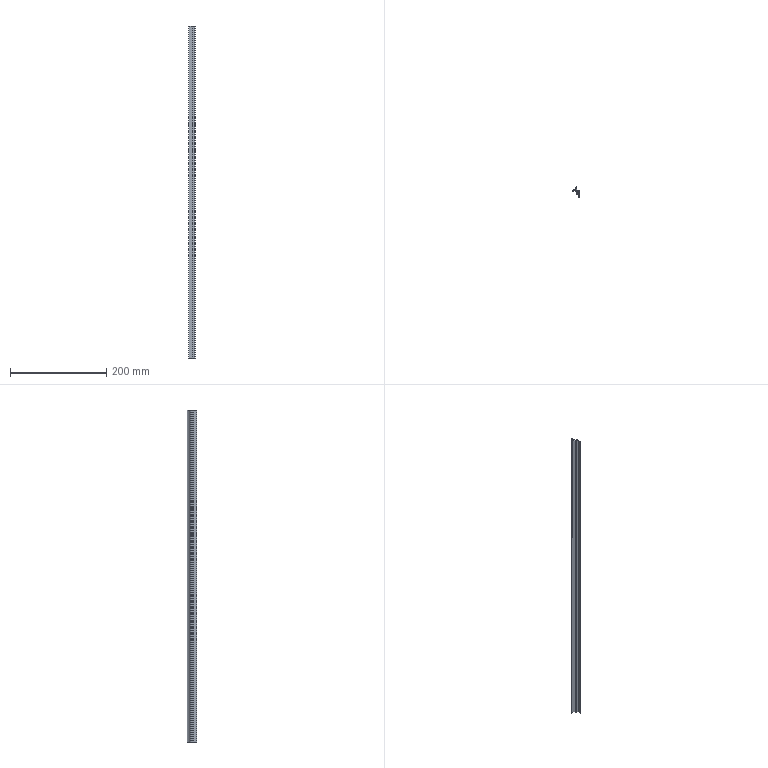Part | SolidWorks | features BaseBody 1, ICE 1, MoveFace 1 | 1 solid | 27 faces | box 14 x 20.3 x 689 mm | volume 35081 mm3 | plane 20 | cylinder 7 | commonest cylinder face diameters 0.387 x2 0.8 x2 0.4 x1 20 x1 22 x1
STEP:
#1=CARTESIAN_POINT('',(-5.304,-0.625,200.));
#2=VERTEX_POINT('',#1);
#3=CARTESIAN_POINT('',(-5.449,-0.8125,200.));
#4=VERTEX_POINT('',#3);
#5=CARTESIAN_POINT('',(-5.255,-0.8125,200.));
#6=DIRECTION('',(0.,0.,1.));
#7=DIRECTION('',(-1.,0.,0.));
#8=AXIS2_PLACEMENT_3D('',#5,#6,#7);
#9=CIRCLE('',#8,0.1937);
#10=EDGE_CURVE('',#2,#4,#9,.T.);
#11=ORIENTED_EDGE('',*,*,#10,.T.);
#12=CARTESIAN_POINT('',(-5.449,-0.8125,-489.));
#13=VERTEX_POINT('',#12);
#14=CARTESIAN_POINT('',(-5.449,-0.8125,230.));
#15=DIRECTION('',(0.,0.,-1.));
#16=VECTOR('',#15,1000.);
#17=LINE('',#14,#16);
#18=EDGE_CURVE('',#4,#13,#17,.T.);
#19=ORIENTED_EDGE('',*,*,#18,.T.);
#20=CARTESIAN_POINT('',(-5.304,-0.625,-489.));
#21=VERTEX_POINT('',#20);
#22=CARTESIAN_POINT('',(-5.255,-0.8125,-489.));
#23=DIRECTION('',(0.,0.,-1.));
#24=DIRECTION('',(1.,0.,0.));
#25=AXIS2_PLACEMENT_3D('',#22,#23,#24);
#26=CIRCLE('',#25,0.1937);
#27=EDGE_CURVE('',#13,#21,#26,.T.);
#28=ORIENTED_EDGE('',*,*,#27,.T.);
#29=CARTESIAN_POINT('',(-5.304,-0.625,230.));
#30=DIRECTION('',(0.,0.,-1.));
#31=VECTOR('',#30,1000.);
#32=LINE('',#29,#31);
#33=EDGE_CURVE('',#2,#21,#32,.T.);
#34=ORIENTED_EDGE('',*,*,#33,.F.);
#35=EDGE_LOOP('',(#11,#19,#28,#34));
#36=FACE_OUTER_BOUND('',#35,.T.);
#37=CARTESIAN_POINT('',(-5.255,-0.8125,230.));
#38=DIRECTION('',(0.,0.,-1.));
#39=DIRECTION('',(-1.,0.,0.));
#40=AXIS2_PLACEMENT_3D('',#37,#38,#39);
#41=CYLINDRICAL_SURFACE('',#40,0.1937);
#42=ADVANCED_FACE('',(#36),#41,.F.);
#43=CARTESIAN_POINT('',(5.,-1.,-489.));
#44=VERTEX_POINT('',#43);
#45=CARTESIAN_POINT('',(5.,-14.3,-489.));
#46=VERTEX_POINT('',#45);
#47=CARTESIAN_POINT('',(5.,29.623,-489.));
#48=DIRECTION('',(0.,-1.,0.));
#49=VECTOR('',#48,1000.);
#50=LINE('',#47,#49);
#51=EDGE_CURVE('',#44,#46,#50,.T.);
#52=ORIENTED_EDGE('',*,*,#51,.F.);
#53=CARTESIAN_POINT('',(5.,-1.,200.));
#54=VERTEX_POINT('',#53);
#55=CARTESIAN_POINT('',(5.,-1.,230.));
#56=DIRECTION('',(0.,0.,-1.));
#57=VECTOR('',#56,1000.);
#58=LINE('',#55,#57);
#59=EDGE_CURVE('',#54,#44,#58,.T.);
#60=ORIENTED_EDGE('',*,*,#59,.F.);
#61=CARTESIAN_POINT('',(5.,-14.3,200.));
#62=VERTEX_POINT('',#61);
#63=CARTESIAN_POINT('',(5.,-14.3,200.));
#64=DIRECTION('',(0.,1.,0.));
#65=VECTOR('',#64,1000.);
#66=LINE('',#63,#65);
#67=EDGE_CURVE('',#62,#54,#66,.T.);
#68=ORIENTED_EDGE('',*,*,#67,.F.);
#69=CARTESIAN_POINT('',(5.,-14.3,230.));
#70=DIRECTION('',(0.,0.,1.));
#71=VECTOR('',#70,1000.);
#72=LINE('',#69,#71);
#73=EDGE_CURVE('',#46,#62,#72,.T.);
#74=ORIENTED_EDGE('',*,*,#73,.F.);
#75=EDGE_LOOP('',(#52,#60,#68,#74));
#76=FACE_OUTER_BOUND('',#75,.T.);
#77=CARTESIAN_POINT('',(5.,-14.3,230.));
#78=DIRECTION('',(-1.,0.,0.));
#79=DIRECTION('',(0.,0.,1.));
#80=AXIS2_PLACEMENT_3D('',#77,#78,#79);
#81=PLANE('',#80);
#82=ADVANCED_FACE('',(#76),#81,.F.);
#83=CARTESIAN_POINT('',(-9.,-2.,-489.));
#84=VERTEX_POINT('',#83);
#85=CARTESIAN_POINT('',(-9.,-2.,200.));
#86=VERTEX_POINT('',#85);
#87=CARTESIAN_POINT('',(-9.,-2.,230.));
#88=DIRECTION('',(0.,0.,1.));
#89=VECTOR('',#88,1000.);
#90=LINE('',#87,#89);
#91=EDGE_CURVE('',#84,#86,#90,.T.);
#92=ORIENTED_EDGE('',*,*,#91,.F.);
#93=CARTESIAN_POINT('',(0.9,-2.,-489.));
#94=VERTEX_POINT('',#93);
#95=CARTESIAN_POINT('',(5.,-2.,-489.));
#96=DIRECTION('',(-1.,0.,0.));
#97=VECTOR('',#96,1000.);
#98=LINE('',#95,#97);
#99=EDGE_CURVE('',#94,#84,#98,.T.);
#100=ORIENTED_EDGE('',*,*,#99,.F.);
#101=CARTESIAN_POINT('',(0.9,-2.,200.));
#102=VERTEX_POINT('',#101);
#103=CARTESIAN_POINT('',(0.9,-2.,230.));
#104=DIRECTION('',(0.,0.,-1.));
#105=VECTOR('',#104,1000.);
#106=LINE('',#103,#105);
#107=EDGE_CURVE('',#102,#94,#106,.T.);
#108=ORIENTED_EDGE('',*,*,#107,.F.);
#109=CARTESIAN_POINT('',(5.,-2.,200.));
#110=DIRECTION('',(1.,0.,0.));
#111=VECTOR('',#110,1000.);
#112=LINE('',#109,#111);
#113=EDGE_CURVE('',#86,#102,#112,.T.);
#114=ORIENTED_EDGE('',*,*,#113,.F.);
#115=EDGE_LOOP('',(#92,#100,#108,#114));
#116=FACE_OUTER_BOUND('',#115,.T.);
#117=CARTESIAN_POINT('',(-9.,-2.,230.));
#118=DIRECTION('',(0.,1.,0.));
#119=DIRECTION('',(0.,0.,1.));
#120=AXIS2_PLACEMENT_3D('',#117,#118,#119);
#121=PLANE('',#120);
#122=ADVANCED_FACE('',(#116),#121,.F.);
#123=CARTESIAN_POINT('',(4.,-6.,200.));
#124=VERTEX_POINT('',#123);
#125=CARTESIAN_POINT('',(4.,-3.,200.));
#126=VERTEX_POINT('',#125);
#127=CARTESIAN_POINT('',(4.,29.623,200.));
#128=DIRECTION('',(0.,1.,0.));
#129=VECTOR('',#128,1000.);
#130=LINE('',#127,#129);
#131=EDGE_CURVE('',#124,#126,#130,.T.);
#132=ORIENTED_EDGE('',*,*,#131,.F.);
#133=CARTESIAN_POINT('',(1.,-6.,200.));
#134=VERTEX_POINT('',#133);
#135=CARTESIAN_POINT('',(5.,-6.,200.));
#136=DIRECTION('',(1.,0.,0.));
#137=VECTOR('',#136,1000.);
#138=LINE('',#135,#137);
#139=EDGE_CURVE('',#134,#124,#138,.T.);
#140=ORIENTED_EDGE('',*,*,#139,.F.);
#141=CARTESIAN_POINT('',(1.,-6.7,200.));
#142=VERTEX_POINT('',#141);
#143=CARTESIAN_POINT('',(1.,-6.,200.));
#144=DIRECTION('',(0.,-1.,0.));
#145=VECTOR('',#144,1000.);
#146=LINE('',#143,#145);
#147=EDGE_CURVE('',#134,#142,#146,.T.);
#148=ORIENTED_EDGE('',*,*,#147,.T.);
#149=CARTESIAN_POINT('',(-1.7,-6.7,200.));
#150=VERTEX_POINT('',#149);
#151=CARTESIAN_POINT('',(5.,-6.7,200.));
#152=DIRECTION('',(1.,0.,0.));
#153=VECTOR('',#152,1000.);
#154=LINE('',#151,#153);
#155=EDGE_CURVE('',#150,#142,#154,.T.);
#156=ORIENTED_EDGE('',*,*,#155,.F.);
#157=CARTESIAN_POINT('',(-1.7,-7.7,200.));
#158=VERTEX_POINT('',#157);
#159=CARTESIAN_POINT('',(-1.7,-6.7,200.));
#160=DIRECTION('',(0.,-1.,0.));
#161=VECTOR('',#160,1000.);
#162=LINE('',#159,#161);
#163=EDGE_CURVE('',#150,#158,#162,.T.);
#164=ORIENTED_EDGE('',*,*,#163,.T.);
#165=CARTESIAN_POINT('',(4.,-7.7,200.));
#166=VERTEX_POINT('',#165);
#167=CARTESIAN_POINT('',(5.,-7.7,200.));
#168=DIRECTION('',(-1.,0.,0.));
#169=VECTOR('',#168,1000.);
#170=LINE('',#167,#169);
#171=EDGE_CURVE('',#166,#158,#170,.T.);
#172=ORIENTED_EDGE('',*,*,#171,.F.);
#173=CARTESIAN_POINT('',(4.,-14.3,200.));
#174=VERTEX_POINT('',#173);
#175=CARTESIAN_POINT('',(4.,29.623,200.));
#176=DIRECTION('',(0.,1.,0.));
#177=VECTOR('',#176,1000.);
#178=LINE('',#175,#177);
#179=EDGE_CURVE('',#174,#166,#178,.T.);
#180=ORIENTED_EDGE('',*,*,#179,.F.);
#181=CARTESIAN_POINT('',(5.,-14.3,200.));
#182=DIRECTION('',(-1.,0.,0.));
#183=VECTOR('',#182,1000.);
#184=LINE('',#181,#183);
#185=EDGE_CURVE('',#62,#174,#184,.T.);
#186=ORIENTED_EDGE('',*,*,#185,.F.);
#187=ORIENTED_EDGE('',*,*,#67,.T.);
#188=CARTESIAN_POINT('',(-5.207,-1.,200.));
#189=VERTEX_POINT('',#188);
#190=CARTESIAN_POINT('',(5.,-1.,200.));
#191=DIRECTION('',(1.,0.,0.));
#192=VECTOR('',#191,1000.);
#193=LINE('',#190,#192);
#194=EDGE_CURVE('',#189,#54,#193,.T.);
#195=ORIENTED_EDGE('',*,*,#194,.F.);
#196=CARTESIAN_POINT('',(-5.255,-0.8125,200.));
#197=DIRECTION('',(0.,0.,1.));
#198=DIRECTION('',(-1.,0.,0.));
#199=AXIS2_PLACEMENT_3D('',#196,#197,#198);
#200=CIRCLE('',#199,0.1937);
#201=EDGE_CURVE('',#4,#189,#200,.T.);
#202=ORIENTED_EDGE('',*,*,#201,.F.);
#203=ORIENTED_EDGE('',*,*,#10,.F.);
#204=CARTESIAN_POINT('',(-1.368,3.063,200.));
#205=VERTEX_POINT('',#204);
#206=CARTESIAN_POINT('',(-10.628,9.,200.));
#207=DIRECTION('',(0.,0.,1.));
#208=DIRECTION('',(-1.,0.,0.));
#209=AXIS2_PLACEMENT_3D('',#206,#207,#208);
#210=CIRCLE('',#209,11.);
#211=EDGE_CURVE('',#2,#205,#210,.T.);
#212=ORIENTED_EDGE('',*,*,#211,.T.);
#213=CARTESIAN_POINT('',(-1.,2.955,200.));
#214=VERTEX_POINT('',#213);
#215=CARTESIAN_POINT('',(-1.2,2.955,200.));
#216=DIRECTION('',(0.,0.,1.));
#217=DIRECTION('',(-1.,0.,0.));
#218=AXIS2_PLACEMENT_3D('',#215,#216,#217);
#219=CIRCLE('',#218,0.2);
#220=EDGE_CURVE('',#214,#205,#219,.T.);
#221=ORIENTED_EDGE('',*,*,#220,.F.);
#222=CARTESIAN_POINT('',(-1.,1.5,200.));
#223=VERTEX_POINT('',#222);
#224=CARTESIAN_POINT('',(-1.,2.955,200.));
#225=DIRECTION('',(0.,1.,0.));
#226=VECTOR('',#225,1000.);
#227=LINE('',#224,#226);
#228=EDGE_CURVE('',#223,#214,#227,.T.);
#229=ORIENTED_EDGE('',*,*,#228,.F.);
#230=CARTESIAN_POINT('',(0.,1.5,200.));
#231=VERTEX_POINT('',#230);
#232=CARTESIAN_POINT('',(-1.,1.5,200.));
#233=DIRECTION('',(-1.,0.,0.));
#234=VECTOR('',#233,1000.);
#235=LINE('',#232,#234);
#236=EDGE_CURVE('',#231,#223,#235,.T.);
#237=ORIENTED_EDGE('',*,*,#236,.F.);
#238=CARTESIAN_POINT('',(0.,6.,200.));
#239=VERTEX_POINT('',#238);
#240=CARTESIAN_POINT('',(0.,1.5,200.));
#241=DIRECTION('',(0.,-1.,0.));
#242=VECTOR('',#241,1000.);
#243=LINE('',#240,#242);
#244=EDGE_CURVE('',#239,#231,#243,.T.);
#245=ORIENTED_EDGE('',*,*,#244,.F.);
#246=CARTESIAN_POINT('',(-0.8,6.,200.));
#247=VERTEX_POINT('',#246);
#248=CARTESIAN_POINT('',(0.,6.,200.));
#249=DIRECTION('',(1.,0.,0.));
#250=VECTOR('',#249,1000.);
#251=LINE('',#248,#250);
#252=EDGE_CURVE('',#247,#239,#251,.T.);
#253=ORIENTED_EDGE('',*,*,#252,.F.);
#254=CARTESIAN_POINT('',(-1.178,5.731,200.));
#255=VERTEX_POINT('',#254);
#256=CARTESIAN_POINT('',(-0.8,5.6,200.));
#257=DIRECTION('',(0.,0.,1.));
#258=DIRECTION('',(-1.,0.,0.));
#259=AXIS2_PLACEMENT_3D('',#256,#257,#258);
#260=CIRCLE('',#259,0.4);
#261=EDGE_CURVE('',#247,#255,#260,.T.);
#262=ORIENTED_EDGE('',*,*,#261,.T.);
#263=CARTESIAN_POINT('',(-8.678,-0.8077,200.));
#264=VERTEX_POINT('',#263);
#265=CARTESIAN_POINT('',(-10.628,9.,200.));
#266=DIRECTION('',(0.,0.,1.));
#267=DIRECTION('',(-1.,0.,0.));
#268=AXIS2_PLACEMENT_3D('',#265,#266,#267);
#269=CIRCLE('',#268,10.);
#270=EDGE_CURVE('',#264,#255,#269,.T.);
#271=ORIENTED_EDGE('',*,*,#270,.F.);
#272=CARTESIAN_POINT('',(-9.,-1.2,200.));
#273=VERTEX_POINT('',#272);
#274=CARTESIAN_POINT('',(-8.6,-1.2,200.));
#275=DIRECTION('',(0.,0.,1.));
#276=DIRECTION('',(-1.,0.,0.));
#277=AXIS2_PLACEMENT_3D('',#274,#275,#276);
#278=CIRCLE('',#277,0.4);
#279=EDGE_CURVE('',#264,#273,#278,.T.);
#280=ORIENTED_EDGE('',*,*,#279,.T.);
#281=CARTESIAN_POINT('',(-9.,8.,200.));
#282=DIRECTION('',(0.,-1.,0.));
#283=VECTOR('',#282,1000.);
#284=LINE('',#281,#283);
#285=EDGE_CURVE('',#273,#86,#284,.T.);
#286=ORIENTED_EDGE('',*,*,#285,.T.);
#287=ORIENTED_EDGE('',*,*,#113,.T.);
#288=CARTESIAN_POINT('',(0.9,-3.,200.));
#289=VERTEX_POINT('',#288);
#290=CARTESIAN_POINT('',(0.9,29.623,200.));
#291=DIRECTION('',(0.,1.,0.));
#292=VECTOR('',#291,1000.);
#293=LINE('',#290,#292);
#294=EDGE_CURVE('',#289,#102,#293,.T.);
#295=ORIENTED_EDGE('',*,*,#294,.F.);
#296=CARTESIAN_POINT('',(5.,-3.,200.));
#297=DIRECTION('',(-1.,0.,0.));
#298=VECTOR('',#297,1000.);
#299=LINE('',#296,#298);
#300=EDGE_CURVE('',#126,#289,#299,.T.);
#301=ORIENTED_EDGE('',*,*,#300,.F.);
#302=EDGE_LOOP('',(#132,#140,#148,#156,#164,#172,#180,#186,#187,#195,#202,#203,#212,#221,#229,#237,#245,#253,#262,#271,#280,#286,#287,#295,#301));
#303=FACE_OUTER_BOUND('',#302,.T.);
#304=CARTESIAN_POINT('',(5.,29.623,200.));
#305=DIRECTION('',(0.,0.,-1.));
#306=DIRECTION('',(-1.,0.,0.));
#307=AXIS2_PLACEMENT_3D('',#304,#305,#306);
#308=PLANE('',#307);
#309=ADVANCED_FACE('',(#303),#308,.F.);
#310=ORIENTED_EDGE('',*,*,#185,.T.);
#311=CARTESIAN_POINT('',(4.,-14.3,-489.));
#312=VERTEX_POINT('',#311);
#313=CARTESIAN_POINT('',(4.,-14.3,230.));
#314=DIRECTION('',(0.,0.,1.));
#315=VECTOR('',#314,1000.);
#316=LINE('',#313,#315);
#317=EDGE_CURVE('',#312,#174,#316,.T.);
#318=ORIENTED_EDGE('',*,*,#317,.F.);
#319=CARTESIAN_POINT('',(5.,-14.3,-489.));
#320=DIRECTION('',(-1.,0.,0.));
#321=VECTOR('',#320,1000.);
#322=LINE('',#319,#321);
#323=EDGE_CURVE('',#46,#312,#322,.T.);
#324=ORIENTED_EDGE('',*,*,#323,.F.);
#325=ORIENTED_EDGE('',*,*,#73,.T.);
#326=EDGE_LOOP('',(#310,#318,#324,#325));
#327=FACE_OUTER_BOUND('',#326,.T.);
#328=CARTESIAN_POINT('',(4.,-14.3,230.));
#329=DIRECTION('',(0.,1.,0.));
#330=DIRECTION('',(0.,0.,1.));
#331=AXIS2_PLACEMENT_3D('',#328,#329,#330);
#332=PLANE('',#331);
#333=ADVANCED_FACE('',(#327),#332,.F.);
#334=ORIENTED_EDGE('',*,*,#51,.T.);
#335=ORIENTED_EDGE('',*,*,#323,.T.);
#336=CARTESIAN_POINT('',(4.,-7.7,-489.));
#337=VERTEX_POINT('',#336);
#338=CARTESIAN_POINT('',(4.,-7.7,-489.));
#339=DIRECTION('',(0.,-1.,0.));
#340=VECTOR('',#339,1000.);
#341=LINE('',#338,#340);
#342=EDGE_CURVE('',#337,#312,#341,.T.);
#343=ORIENTED_EDGE('',*,*,#342,.F.);
#344=CARTESIAN_POINT('',(-1.7,-7.7,-489.));
#345=VERTEX_POINT('',#344);
#346=CARTESIAN_POINT('',(-1.7,-7.7,-489.));
#347=DIRECTION('',(1.,0.,0.));
#348=VECTOR('',#347,1000.);
#349=LINE('',#346,#348);
#350=EDGE_CURVE('',#345,#337,#349,.T.);
#351=ORIENTED_EDGE('',*,*,#350,.F.);
#352=CARTESIAN_POINT('',(-1.7,-6.7,-489.));
#353=VERTEX_POINT('',#352);
#354=CARTESIAN_POINT('',(-1.7,29.623,-489.));
#355=DIRECTION('',(0.,1.,0.));
#356=VECTOR('',#355,1000.);
#357=LINE('',#354,#356);
#358=EDGE_CURVE('',#345,#353,#357,.T.);
#359=ORIENTED_EDGE('',*,*,#358,.T.);
#360=CARTESIAN_POINT('',(1.,-6.7,-489.));
#361=VERTEX_POINT('',#360);
#362=CARTESIAN_POINT('',(1.,-6.7,-489.));
#363=DIRECTION('',(-1.,0.,0.));
#364=VECTOR('',#363,1000.);
#365=LINE('',#362,#364);
#366=EDGE_CURVE('',#361,#353,#365,.T.);
#367=ORIENTED_EDGE('',*,*,#366,.F.);
#368=CARTESIAN_POINT('',(1.,-6.,-489.));
#369=VERTEX_POINT('',#368);
#370=CARTESIAN_POINT('',(1.,29.623,-489.));
#371=DIRECTION('',(0.,1.,0.));
#372=VECTOR('',#371,1000.);
#373=LINE('',#370,#372);
#374=EDGE_CURVE('',#361,#369,#373,.T.);
#375=ORIENTED_EDGE('',*,*,#374,.T.);
#376=CARTESIAN_POINT('',(4.,-6.,-489.));
#377=VERTEX_POINT('',#376);
#378=CARTESIAN_POINT('',(4.,-6.,-489.));
#379=DIRECTION('',(-1.,0.,0.));
#380=VECTOR('',#379,1000.);
#381=LINE('',#378,#380);
#382=EDGE_CURVE('',#377,#369,#381,.T.);
#383=ORIENTED_EDGE('',*,*,#382,.F.);
#384=CARTESIAN_POINT('',(4.,-3.,-489.));
#385=VERTEX_POINT('',#384);
#386=CARTESIAN_POINT('',(4.,-3.,-489.));
#387=DIRECTION('',(0.,-1.,0.));
#388=VECTOR('',#387,1000.);
#389=LINE('',#386,#388);
#390=EDGE_CURVE('',#385,#377,#389,.T.);
#391=ORIENTED_EDGE('',*,*,#390,.F.);
#392=CARTESIAN_POINT('',(0.9,-3.,-489.));
#393=VERTEX_POINT('',#392);
#394=CARTESIAN_POINT('',(0.9,-3.,-489.));
#395=DIRECTION('',(1.,0.,0.));
#396=VECTOR('',#395,1000.);
#397=LINE('',#394,#396);
#398=EDGE_CURVE('',#393,#385,#397,.T.);
#399=ORIENTED_EDGE('',*,*,#398,.F.);
#400=CARTESIAN_POINT('',(0.9,-2.,-489.));
#401=DIRECTION('',(0.,-1.,0.));
#402=VECTOR('',#401,1000.);
#403=LINE('',#400,#402);
#404=EDGE_CURVE('',#94,#393,#403,.T.);
#405=ORIENTED_EDGE('',*,*,#404,.F.);
#406=ORIENTED_EDGE('',*,*,#99,.T.);
#407=CARTESIAN_POINT('',(-9.,-1.2,-489.));
#408=VERTEX_POINT('',#407);
#409=CARTESIAN_POINT('',(-9.,-1.2,-489.));
#410=DIRECTION('',(0.,-1.,0.));
#411=VECTOR('',#410,1000.);
#412=LINE('',#409,#411);
#413=EDGE_CURVE('',#408,#84,#412,.T.);
#414=ORIENTED_EDGE('',*,*,#413,.F.);
#415=CARTESIAN_POINT('',(-8.678,-0.8077,-489.));
#416=VERTEX_POINT('',#415);
#417=CARTESIAN_POINT('',(-8.6,-1.2,-489.));
#418=DIRECTION('',(0.,0.,-1.));
#419=DIRECTION('',(1.,0.,0.));
#420=AXIS2_PLACEMENT_3D('',#417,#418,#419);
#421=CIRCLE('',#420,0.4);
#422=EDGE_CURVE('',#408,#416,#421,.T.);
#423=ORIENTED_EDGE('',*,*,#422,.T.);
#424=CARTESIAN_POINT('',(-1.178,5.731,-489.));
#425=VERTEX_POINT('',#424);
#426=CARTESIAN_POINT('',(-10.628,9.,-489.));
#427=DIRECTION('',(0.,0.,-1.));
#428=DIRECTION('',(1.,0.,0.));
#429=AXIS2_PLACEMENT_3D('',#426,#427,#428);
#430=CIRCLE('',#429,10.);
#431=EDGE_CURVE('',#425,#416,#430,.T.);
#432=ORIENTED_EDGE('',*,*,#431,.F.);
#433=CARTESIAN_POINT('',(-0.8,6.,-489.));
#434=VERTEX_POINT('',#433);
#435=CARTESIAN_POINT('',(-0.8,5.6,-489.));
#436=DIRECTION('',(0.,0.,-1.));
#437=DIRECTION('',(1.,0.,0.));
#438=AXIS2_PLACEMENT_3D('',#435,#436,#437);
#439=CIRCLE('',#438,0.4);
#440=EDGE_CURVE('',#425,#434,#439,.T.);
#441=ORIENTED_EDGE('',*,*,#440,.T.);
#442=CARTESIAN_POINT('',(0.,6.,-489.));
#443=VERTEX_POINT('',#442);
#444=CARTESIAN_POINT('',(0.,6.,-489.));
#445=DIRECTION('',(-1.,0.,0.));
#446=VECTOR('',#445,1000.);
#447=LINE('',#444,#446);
#448=EDGE_CURVE('',#443,#434,#447,.T.);
#449=ORIENTED_EDGE('',*,*,#448,.F.);
#450=CARTESIAN_POINT('',(0.,1.5,-489.));
#451=VERTEX_POINT('',#450);
#452=CARTESIAN_POINT('',(0.,1.5,-489.));
#453=DIRECTION('',(0.,1.,0.));
#454=VECTOR('',#453,1000.);
#455=LINE('',#452,#454);
#456=EDGE_CURVE('',#451,#443,#455,.T.);
#457=ORIENTED_EDGE('',*,*,#456,.F.);
#458=CARTESIAN_POINT('',(-1.,1.5,-489.));
#459=VERTEX_POINT('',#458);
#460=CARTESIAN_POINT('',(-1.,1.5,-489.));
#461=DIRECTION('',(1.,0.,0.));
#462=VECTOR('',#461,1000.);
#463=LINE('',#460,#462);
#464=EDGE_CURVE('',#459,#451,#463,.T.);
#465=ORIENTED_EDGE('',*,*,#464,.F.);
#466=CARTESIAN_POINT('',(-1.,2.955,-489.));
#467=VERTEX_POINT('',#466);
#468=CARTESIAN_POINT('',(-1.,2.955,-489.));
#469=DIRECTION('',(0.,-1.,0.));
#470=VECTOR('',#469,1000.);
#471=LINE('',#468,#470);
#472=EDGE_CURVE('',#467,#459,#471,.T.);
#473=ORIENTED_EDGE('',*,*,#472,.F.);
#474=CARTESIAN_POINT('',(-1.368,3.063,-489.));
#475=VERTEX_POINT('',#474);
#476=CARTESIAN_POINT('',(-1.2,2.955,-489.));
#477=DIRECTION('',(0.,0.,-1.));
#478=DIRECTION('',(1.,0.,0.));
#479=AXIS2_PLACEMENT_3D('',#476,#477,#478);
#480=CIRCLE('',#479,0.2);
#481=EDGE_CURVE('',#475,#467,#480,.T.);
#482=ORIENTED_EDGE('',*,*,#481,.F.);
#483=CARTESIAN_POINT('',(-10.628,9.,-489.));
#484=DIRECTION('',(0.,0.,-1.));
#485=DIRECTION('',(1.,0.,0.));
#486=AXIS2_PLACEMENT_3D('',#483,#484,#485);
#487=CIRCLE('',#486,11.);
#488=EDGE_CURVE('',#475,#21,#487,.T.);
#489=ORIENTED_EDGE('',*,*,#488,.T.);
#490=ORIENTED_EDGE('',*,*,#27,.F.);
#491=CARTESIAN_POINT('',(-5.207,-1.,-489.));
#492=VERTEX_POINT('',#491);
#493=CARTESIAN_POINT('',(-5.255,-0.8125,-489.));
#494=DIRECTION('',(0.,0.,-1.));
#495=DIRECTION('',(1.,0.,0.));
#496=AXIS2_PLACEMENT_3D('',#493,#494,#495);
#497=CIRCLE('',#496,0.1937);
#498=EDGE_CURVE('',#492,#13,#497,.T.);
#499=ORIENTED_EDGE('',*,*,#498,.F.);
#500=CARTESIAN_POINT('',(5.,-1.,-489.));
#501=DIRECTION('',(-1.,0.,0.));
#502=VECTOR('',#501,1000.);
#503=LINE('',#500,#502);
#504=EDGE_CURVE('',#44,#492,#503,.T.);
#505=ORIENTED_EDGE('',*,*,#504,.F.);
#506=EDGE_LOOP('',(#334,#335,#343,#351,#359,#367,#375,#383,#391,#399,#405,#406,#414,#423,#432,#441,#449,#457,#465,#473,#482,#489,#490,#499,#505));
#507=FACE_OUTER_BOUND('',#506,.T.);
#508=CARTESIAN_POINT('',(5.,29.623,-489.));
#509=DIRECTION('',(0.,0.,1.));
#510=DIRECTION('',(1.,0.,0.));
#511=AXIS2_PLACEMENT_3D('',#508,#509,#510);
#512=PLANE('',#511);
#513=ADVANCED_FACE('',(#507),#512,.F.);
#514=ORIENTED_EDGE('',*,*,#59,.T.);
#515=ORIENTED_EDGE('',*,*,#504,.T.);
#516=CARTESIAN_POINT('',(-5.207,-1.,230.));
#517=DIRECTION('',(0.,0.,-1.));
#518=VECTOR('',#517,1000.);
#519=LINE('',#516,#518);
#520=EDGE_CURVE('',#189,#492,#519,.T.);
#521=ORIENTED_EDGE('',*,*,#520,.F.);
#522=ORIENTED_EDGE('',*,*,#194,.T.);
#523=EDGE_LOOP('',(#514,#515,#521,#522));
#524=FACE_OUTER_BOUND('',#523,.T.);
#525=CARTESIAN_POINT('',(5.,-1.,230.));
#526=DIRECTION('',(0.,-1.,0.));
#527=DIRECTION('',(0.,0.,-1.));
#528=AXIS2_PLACEMENT_3D('',#525,#526,#527);
#529=PLANE('',#528);
#530=ADVANCED_FACE('',(#524),#529,.F.);
#531=CARTESIAN_POINT('',(-9.,-1.2,230.));
#532=DIRECTION('',(0.,0.,1.));
#533=VECTOR('',#532,1000.);
#534=LINE('',#531,#533);
#535=EDGE_CURVE('',#408,#273,#534,.T.);
#536=ORIENTED_EDGE('',*,*,#535,.F.);
#537=ORIENTED_EDGE('',*,*,#413,.T.);
#538=ORIENTED_EDGE('',*,*,#91,.T.);
#539=ORIENTED_EDGE('',*,*,#285,.F.);
#540=EDGE_LOOP('',(#536,#537,#538,#539));
#541=FACE_OUTER_BOUND('',#540,.T.);
#542=CARTESIAN_POINT('',(-9.,-1.2,230.));
#543=DIRECTION('',(1.,0.,0.));
#544=DIRECTION('',(0.,0.,-1.));
#545=AXIS2_PLACEMENT_3D('',#542,#543,#544);
#546=PLANE('',#545);
#547=ADVANCED_FACE('',(#541),#546,.F.);
#548=ORIENTED_EDGE('',*,*,#294,.T.);
#549=ORIENTED_EDGE('',*,*,#107,.T.);
#550=ORIENTED_EDGE('',*,*,#404,.T.);
#551=CARTESIAN_POINT('',(0.9,-3.,230.));
#552=DIRECTION('',(0.,0.,-1.));
#553=VECTOR('',#552,1000.);
#554=LINE('',#551,#553);
#555=EDGE_CURVE('',#289,#393,#554,.T.);
#556=ORIENTED_EDGE('',*,*,#555,.F.);
#557=EDGE_LOOP('',(#548,#549,#550,#556));
#558=FACE_OUTER_BOUND('',#557,.T.);
#559=CARTESIAN_POINT('',(0.9,-2.,230.));
#560=DIRECTION('',(1.,0.,0.));
#561=DIRECTION('',(0.,0.,-1.));
#562=AXIS2_PLACEMENT_3D('',#559,#560,#561);
#563=PLANE('',#562);
#564=ADVANCED_FACE('',(#558),#563,.F.);
#565=ORIENTED_EDGE('',*,*,#300,.T.);
#566=ORIENTED_EDGE('',*,*,#555,.T.);
#567=ORIENTED_EDGE('',*,*,#398,.T.);
#568=CARTESIAN_POINT('',(4.,-3.,230.));
#569=DIRECTION('',(0.,0.,-1.));
#570=VECTOR('',#569,1000.);
#571=LINE('',#568,#570);
#572=EDGE_CURVE('',#126,#385,#571,.T.);
#573=ORIENTED_EDGE('',*,*,#572,.F.);
#574=EDGE_LOOP('',(#565,#566,#567,#573));
#575=FACE_OUTER_BOUND('',#574,.T.);
#576=CARTESIAN_POINT('',(0.9,-3.,230.));
#577=DIRECTION('',(0.,1.,0.));
#578=DIRECTION('',(0.,0.,1.));
#579=AXIS2_PLACEMENT_3D('',#576,#577,#578);
#580=PLANE('',#579);
#581=ADVANCED_FACE('',(#575),#580,.F.);
#582=ORIENTED_EDGE('',*,*,#131,.T.);
#583=ORIENTED_EDGE('',*,*,#572,.T.);
#584=ORIENTED_EDGE('',*,*,#390,.T.);
#585=CARTESIAN_POINT('',(4.,-6.,230.));
#586=DIRECTION('',(0.,0.,-1.));
#587=VECTOR('',#586,1000.);
#588=LINE('',#585,#587);
#589=EDGE_CURVE('',#124,#377,#588,.T.);
#590=ORIENTED_EDGE('',*,*,#589,.F.);
#591=EDGE_LOOP('',(#582,#583,#584,#590));
#592=FACE_OUTER_BOUND('',#591,.T.);
#593=CARTESIAN_POINT('',(4.,-3.,230.));
#594=DIRECTION('',(1.,0.,0.));
#595=DIRECTION('',(0.,0.,-1.));
#596=AXIS2_PLACEMENT_3D('',#593,#594,#595);
#597=PLANE('',#596);
#598=ADVANCED_FACE('',(#592),#597,.F.);
#599=ORIENTED_EDGE('',*,*,#139,.T.);
#600=ORIENTED_EDGE('',*,*,#589,.T.);
#601=ORIENTED_EDGE('',*,*,#382,.T.);
#602=CARTESIAN_POINT('',(1.,-6.,230.));
#603=DIRECTION('',(0.,0.,-1.));
#604=VECTOR('',#603,1000.);
#605=LINE('',#602,#604);
#606=EDGE_CURVE('',#134,#369,#605,.T.);
#607=ORIENTED_EDGE('',*,*,#606,.F.);
#608=EDGE_LOOP('',(#599,#600,#601,#607));
#609=FACE_OUTER_BOUND('',#608,.T.);
#610=CARTESIAN_POINT('',(4.,-6.,230.));
#611=DIRECTION('',(0.,-1.,0.));
#612=DIRECTION('',(0.,0.,-1.));
#613=AXIS2_PLACEMENT_3D('',#610,#611,#612);
#614=PLANE('',#613);
#615=ADVANCED_FACE('',(#609),#614,.F.);
#616=ORIENTED_EDGE('',*,*,#155,.T.);
#617=CARTESIAN_POINT('',(1.,-6.7,230.));
#618=DIRECTION('',(0.,0.,1.));
#619=VECTOR('',#618,1000.);
#620=LINE('',#617,#619);
#621=EDGE_CURVE('',#361,#142,#620,.T.);
#622=ORIENTED_EDGE('',*,*,#621,.F.);
#623=ORIENTED_EDGE('',*,*,#366,.T.);
#624=CARTESIAN_POINT('',(-1.7,-6.7,230.));
#625=DIRECTION('',(0.,0.,-1.));
#626=VECTOR('',#625,1000.);
#627=LINE('',#624,#626);
#628=EDGE_CURVE('',#150,#353,#627,.T.);
#629=ORIENTED_EDGE('',*,*,#628,.F.);
#630=EDGE_LOOP('',(#616,#622,#623,#629));
#631=FACE_OUTER_BOUND('',#630,.T.);
#632=CARTESIAN_POINT('',(1.,-6.7,230.));
#633=DIRECTION('',(0.,-1.,0.));
#634=DIRECTION('',(0.,0.,-1.));
#635=AXIS2_PLACEMENT_3D('',#632,#633,#634);
#636=PLANE('',#635);
#637=ADVANCED_FACE('',(#631),#636,.F.);
#638=ORIENTED_EDGE('',*,*,#171,.T.);
#639=CARTESIAN_POINT('',(-1.7,-7.7,230.));
#640=DIRECTION('',(0.,0.,1.));
#641=VECTOR('',#640,1000.);
#642=LINE('',#639,#641);
#643=EDGE_CURVE('',#345,#158,#642,.T.);
#644=ORIENTED_EDGE('',*,*,#643,.F.);
#645=ORIENTED_EDGE('',*,*,#350,.T.);
#646=CARTESIAN_POINT('',(4.,-7.7,230.));
#647=DIRECTION('',(0.,0.,-1.));
#648=VECTOR('',#647,1000.);
#649=LINE('',#646,#648);
#650=EDGE_CURVE('',#166,#337,#649,.T.);
#651=ORIENTED_EDGE('',*,*,#650,.F.);
#652=EDGE_LOOP('',(#638,#644,#645,#651));
#653=FACE_OUTER_BOUND('',#652,.T.);
#654=CARTESIAN_POINT('',(-1.7,-7.7,230.));
#655=DIRECTION('',(0.,1.,0.));
#656=DIRECTION('',(0.,0.,1.));
#657=AXIS2_PLACEMENT_3D('',#654,#655,#656);
#658=PLANE('',#657);
#659=ADVANCED_FACE('',(#653),#658,.F.);
#660=ORIENTED_EDGE('',*,*,#179,.T.);
#661=ORIENTED_EDGE('',*,*,#650,.T.);
#662=ORIENTED_EDGE('',*,*,#342,.T.);
#663=ORIENTED_EDGE('',*,*,#317,.T.);
#664=EDGE_LOOP('',(#660,#661,#662,#663));
#665=FACE_OUTER_BOUND('',#664,.T.);
#666=CARTESIAN_POINT('',(4.,-7.7,230.));
#667=DIRECTION('',(1.,0.,0.));
#668=DIRECTION('',(0.,0.,-1.));
#669=AXIS2_PLACEMENT_3D('',#666,#667,#668);
#670=PLANE('',#669);
#671=ADVANCED_FACE('',(#665),#670,.F.);
#672=ORIENTED_EDGE('',*,*,#18,.F.);
#673=ORIENTED_EDGE('',*,*,#201,.T.);
#674=ORIENTED_EDGE('',*,*,#520,.T.);
#675=ORIENTED_EDGE('',*,*,#498,.T.);
#676=EDGE_LOOP('',(#672,#673,#674,#675));
#677=FACE_OUTER_BOUND('',#676,.T.);
#678=CARTESIAN_POINT('',(-5.255,-0.8125,230.));
#679=DIRECTION('',(0.,0.,-1.));
#680=DIRECTION('',(-1.,0.,0.));
#681=AXIS2_PLACEMENT_3D('',#678,#679,#680);
#682=CYLINDRICAL_SURFACE('',#681,0.1937);
#683=ADVANCED_FACE('',(#677),#682,.F.);
#684=CARTESIAN_POINT('',(-1.,2.955,230.));
#685=DIRECTION('',(0.,0.,1.));
#686=VECTOR('',#685,1000.);
#687=LINE('',#684,#686);
#688=EDGE_CURVE('',#467,#214,#687,.T.);
#689=ORIENTED_EDGE('',*,*,#688,.F.);
#690=ORIENTED_EDGE('',*,*,#472,.T.);
#691=CARTESIAN_POINT('',(-1.,1.5,230.));
#692=DIRECTION('',(0.,0.,-1.));
#693=VECTOR('',#692,1000.);
#694=LINE('',#691,#693);
#695=EDGE_CURVE('',#223,#459,#694,.T.);
#696=ORIENTED_EDGE('',*,*,#695,.F.);
#697=ORIENTED_EDGE('',*,*,#228,.T.);
#698=EDGE_LOOP('',(#689,#690,#696,#697));
#699=FACE_OUTER_BOUND('',#698,.T.);
#700=CARTESIAN_POINT('',(-1.,2.955,230.));
#701=DIRECTION('',(1.,0.,0.));
#702=DIRECTION('',(0.,0.,-1.));
#703=AXIS2_PLACEMENT_3D('',#700,#701,#702);
#704=PLANE('',#703);
#705=ADVANCED_FACE('',(#699),#704,.F.);
#706=ORIENTED_EDGE('',*,*,#488,.F.);
#707=CARTESIAN_POINT('',(-1.368,3.063,230.));
#708=DIRECTION('',(0.,0.,1.));
#709=VECTOR('',#708,1000.);
#710=LINE('',#707,#709);
#711=EDGE_CURVE('',#475,#205,#710,.T.);
#712=ORIENTED_EDGE('',*,*,#711,.T.);
#713=ORIENTED_EDGE('',*,*,#211,.F.);
#714=ORIENTED_EDGE('',*,*,#33,.T.);
#715=EDGE_LOOP('',(#706,#712,#713,#714));
#716=FACE_OUTER_BOUND('',#715,.T.);
#717=CARTESIAN_POINT('',(-10.628,9.,230.));
#718=DIRECTION('',(0.,0.,-1.));
#719=DIRECTION('',(-1.,0.,0.));
#720=AXIS2_PLACEMENT_3D('',#717,#718,#719);
#721=CYLINDRICAL_SURFACE('',#720,11.);
#722=ADVANCED_FACE('',(#716),#721,.T.);
#723=CARTESIAN_POINT('',(-1.178,5.731,230.));
#724=DIRECTION('',(0.,0.,1.));
#725=VECTOR('',#724,1000.);
#726=LINE('',#723,#725);
#727=EDGE_CURVE('',#425,#255,#726,.T.);
#728=ORIENTED_EDGE('',*,*,#727,.F.);
#729=ORIENTED_EDGE('',*,*,#431,.T.);
#730=CARTESIAN_POINT('',(-8.678,-0.8077,230.));
#731=DIRECTION('',(0.,0.,-1.));
#732=VECTOR('',#731,1000.);
#733=LINE('',#730,#732);
#734=EDGE_CURVE('',#264,#416,#733,.T.);
#735=ORIENTED_EDGE('',*,*,#734,.F.);
#736=ORIENTED_EDGE('',*,*,#270,.T.);
#737=EDGE_LOOP('',(#728,#729,#735,#736));
#738=FACE_OUTER_BOUND('',#737,.T.);
#739=CARTESIAN_POINT('',(-10.628,9.,230.));
#740=DIRECTION('',(0.,0.,-1.));
#741=DIRECTION('',(-1.,0.,0.));
#742=AXIS2_PLACEMENT_3D('',#739,#740,#741);
#743=CYLINDRICAL_SURFACE('',#742,10.);
#744=ADVANCED_FACE('',(#738),#743,.F.);
#745=CARTESIAN_POINT('',(0.,1.5,230.));
#746=DIRECTION('',(0.,0.,1.));
#747=VECTOR('',#746,1000.);
#748=LINE('',#745,#747);
#749=EDGE_CURVE('',#451,#231,#748,.T.);
#750=ORIENTED_EDGE('',*,*,#749,.F.);
#751=ORIENTED_EDGE('',*,*,#456,.T.);
#752=CARTESIAN_POINT('',(0.,6.,230.));
#753=DIRECTION('',(0.,0.,-1.));
#754=VECTOR('',#753,1000.);
#755=LINE('',#752,#754);
#756=EDGE_CURVE('',#239,#443,#755,.T.);
#757=ORIENTED_EDGE('',*,*,#756,.F.);
#758=ORIENTED_EDGE('',*,*,#244,.T.);
#759=EDGE_LOOP('',(#750,#751,#757,#758));
#760=FACE_OUTER_BOUND('',#759,.T.);
#761=CARTESIAN_POINT('',(0.,1.5,230.));
#762=DIRECTION('',(-1.,0.,0.));
#763=DIRECTION('',(0.,0.,1.));
#764=AXIS2_PLACEMENT_3D('',#761,#762,#763);
#765=PLANE('',#764);
#766=ADVANCED_FACE('',(#760),#765,.F.);
#767=ORIENTED_EDGE('',*,*,#422,.F.);
#768=ORIENTED_EDGE('',*,*,#535,.T.);
#769=ORIENTED_EDGE('',*,*,#279,.F.);
#770=ORIENTED_EDGE('',*,*,#734,.T.);
#771=EDGE_LOOP('',(#767,#768,#769,#770));
#772=FACE_OUTER_BOUND('',#771,.T.);
#773=CARTESIAN_POINT('',(-8.6,-1.2,230.));
#774=DIRECTION('',(0.,0.,-1.));
#775=DIRECTION('',(-1.,0.,0.));
#776=AXIS2_PLACEMENT_3D('',#773,#774,#775);
#777=CYLINDRICAL_SURFACE('',#776,0.4);
#778=ADVANCED_FACE('',(#772),#777,.T.);
#779=ORIENTED_EDGE('',*,*,#147,.F.);
#780=ORIENTED_EDGE('',*,*,#606,.T.);
#781=ORIENTED_EDGE('',*,*,#374,.F.);
#782=ORIENTED_EDGE('',*,*,#621,.T.);
#783=EDGE_LOOP('',(#779,#780,#781,#782));
#784=FACE_OUTER_BOUND('',#783,.T.);
#785=CARTESIAN_POINT('',(1.,-6.,230.));
#786=DIRECTION('',(1.,0.,0.));
#787=DIRECTION('',(0.,0.,-1.));
#788=AXIS2_PLACEMENT_3D('',#785,#786,#787);
#789=PLANE('',#788);
#790=ADVANCED_FACE('',(#784),#789,.F.);
#791=ORIENTED_EDGE('',*,*,#163,.F.);
#792=ORIENTED_EDGE('',*,*,#628,.T.);
#793=ORIENTED_EDGE('',*,*,#358,.F.);
#794=ORIENTED_EDGE('',*,*,#643,.T.);
#795=EDGE_LOOP('',(#791,#792,#793,#794));
#796=FACE_OUTER_BOUND('',#795,.T.);
#797=CARTESIAN_POINT('',(-1.7,-6.7,230.));
#798=DIRECTION('',(1.,0.,0.));
#799=DIRECTION('',(0.,0.,-1.));
#800=AXIS2_PLACEMENT_3D('',#797,#798,#799);
#801=PLANE('',#800);
#802=ADVANCED_FACE('',(#796),#801,.F.);
#803=ORIENTED_EDGE('',*,*,#711,.F.);
#804=ORIENTED_EDGE('',*,*,#481,.T.);
#805=ORIENTED_EDGE('',*,*,#688,.T.);
#806=ORIENTED_EDGE('',*,*,#220,.T.);
#807=EDGE_LOOP('',(#803,#804,#805,#806));
#808=FACE_OUTER_BOUND('',#807,.T.);
#809=CARTESIAN_POINT('',(-1.2,2.955,230.));
#810=DIRECTION('',(0.,0.,-1.));
#811=DIRECTION('',(-1.,0.,0.));
#812=AXIS2_PLACEMENT_3D('',#809,#810,#811);
#813=CYLINDRICAL_SURFACE('',#812,0.2);
#814=ADVANCED_FACE('',(#808),#813,.F.);
#815=ORIENTED_EDGE('',*,*,#695,.T.);
#816=ORIENTED_EDGE('',*,*,#464,.T.);
#817=ORIENTED_EDGE('',*,*,#749,.T.);
#818=ORIENTED_EDGE('',*,*,#236,.T.);
#819=EDGE_LOOP('',(#815,#816,#817,#818));
#820=FACE_OUTER_BOUND('',#819,.T.);
#821=CARTESIAN_POINT('',(-1.,1.5,230.));
#822=DIRECTION('',(0.,1.,0.));
#823=DIRECTION('',(0.,0.,1.));
#824=AXIS2_PLACEMENT_3D('',#821,#822,#823);
#825=PLANE('',#824);
#826=ADVANCED_FACE('',(#820),#825,.F.);
#827=ORIENTED_EDGE('',*,*,#440,.F.);
#828=ORIENTED_EDGE('',*,*,#727,.T.);
#829=ORIENTED_EDGE('',*,*,#261,.F.);
#830=CARTESIAN_POINT('',(-0.8,6.,230.));
#831=DIRECTION('',(0.,0.,-1.));
#832=VECTOR('',#831,1000.);
#833=LINE('',#830,#832);
#834=EDGE_CURVE('',#247,#434,#833,.T.);
#835=ORIENTED_EDGE('',*,*,#834,.T.);
#836=EDGE_LOOP('',(#827,#828,#829,#835));
#837=FACE_OUTER_BOUND('',#836,.T.);
#838=CARTESIAN_POINT('',(-0.8,5.6,230.));
#839=DIRECTION('',(0.,0.,-1.));
#840=DIRECTION('',(-1.,0.,0.));
#841=AXIS2_PLACEMENT_3D('',#838,#839,#840);
#842=CYLINDRICAL_SURFACE('',#841,0.4);
#843=ADVANCED_FACE('',(#837),#842,.T.);
#844=ORIENTED_EDGE('',*,*,#756,.T.);
#845=ORIENTED_EDGE('',*,*,#448,.T.);
#846=ORIENTED_EDGE('',*,*,#834,.F.);
#847=ORIENTED_EDGE('',*,*,#252,.T.);
#848=EDGE_LOOP('',(#844,#845,#846,#847));
#849=FACE_OUTER_BOUND('',#848,.T.);
#850=CARTESIAN_POINT('',(0.,6.,230.));
#851=DIRECTION('',(0.,-1.,0.));
#852=DIRECTION('',(0.,0.,-1.));
#853=AXIS2_PLACEMENT_3D('',#850,#851,#852);
#854=PLANE('',#853);
#855=ADVANCED_FACE('',(#849),#854,.F.);
#856=CLOSED_SHELL('',(#42,#82,#122,#309,#333,#513,#530,#547,#564,#581,#598,#615,#637,#659,#671,#683,#705,#722,#744,#766,#778,#790,#802,#814,#826,#843,#855));
#857=MANIFOLD_SOLID_BREP('',#856);
#858=CARTESIAN_POINT('',(0.,0.,0.));
#859=DIRECTION('',(0.,0.,1.));
#860=DIRECTION('',(1.,0.,0.));
#861=AXIS2_PLACEMENT_3D('',#858,#859,#860);
#862=(LENGTH_UNIT()NAMED_UNIT(*)SI_UNIT(.MILLI.,.METRE.));
#863=UNCERTAINTY_MEASURE_WITH_UNIT(LENGTH_MEASURE(0.00001),#862,'','');
#864=(NAMED_UNIT(*)PLANE_ANGLE_UNIT()SI_UNIT($,.RADIAN.));
#865=(NAMED_UNIT(*)SI_UNIT($,.STERADIAN.)SOLID_ANGLE_UNIT());
#866=(GEOMETRIC_REPRESENTATION_CONTEXT(3)GLOBAL_UNCERTAINTY_ASSIGNED_CONTEXT((#863))GLOBAL_UNIT_ASSIGNED_CONTEXT((#862,#864,#865))REPRESENTATION_CONTEXT('',''));
#867=ADVANCED_BREP_SHAPE_REPRESENTATION('',(#857,#861),#866);